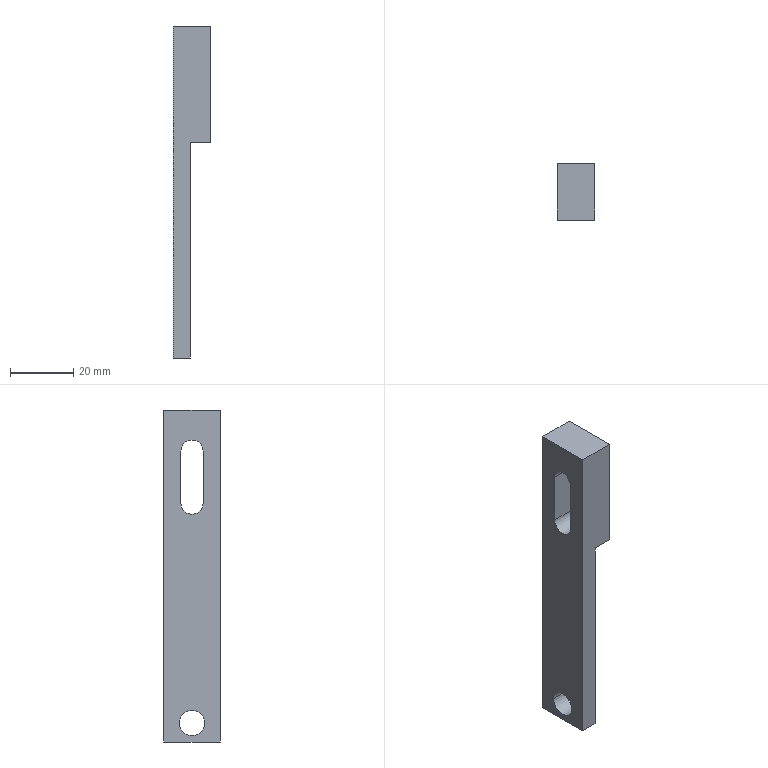Part | NX | 1 solid | 14 faces | box 12 x 18 x 105 mm | volume 12588 mm3 | plane 10 | cylinder 4 | commonest cylinder face diameters 7 x2 8 x2
STEP:
#1=CARTESIAN_POINT('',(-203.,42.75,26.5));
#2=VERTEX_POINT('',#1);
#3=CARTESIAN_POINT('',(-203.,60.75,26.5));
#4=VERTEX_POINT('',#3);
#5=CARTESIAN_POINT('',(-203.,53.935,26.5));
#6=DIRECTION('',(0.,1.,0.));
#7=VECTOR('',#6,1000.);
#8=LINE('',#5,#7);
#9=EDGE_CURVE('',#2,#4,#8,.T.);
#10=ORIENTED_EDGE('',*,*,#9,.T.);
#11=CARTESIAN_POINT('',(-215.,60.75,26.5));
#12=VERTEX_POINT('',#11);
#13=CARTESIAN_POINT('',(-203.,60.75,26.5));
#14=DIRECTION('',(1.,0.,0.));
#15=VECTOR('',#14,1000.);
#16=LINE('',#13,#15);
#17=EDGE_CURVE('',#12,#4,#16,.T.);
#18=ORIENTED_EDGE('',*,*,#17,.F.);
#19=CARTESIAN_POINT('',(-215.,42.75,26.5));
#20=VERTEX_POINT('',#19);
#21=CARTESIAN_POINT('',(-215.,53.935,26.5));
#22=DIRECTION('',(0.,-1.,0.));
#23=VECTOR('',#22,1000.);
#24=LINE('',#21,#23);
#25=EDGE_CURVE('',#12,#20,#24,.T.);
#26=ORIENTED_EDGE('',*,*,#25,.T.);
#27=CARTESIAN_POINT('',(-203.,42.75,26.5));
#28=DIRECTION('',(-1.,0.,0.));
#29=VECTOR('',#28,1000.);
#30=LINE('',#27,#29);
#31=EDGE_CURVE('',#2,#20,#30,.T.);
#32=ORIENTED_EDGE('',*,*,#31,.F.);
#33=EDGE_LOOP('',(#10,#18,#26,#32));
#34=FACE_BOUND('',#33,.T.);
#35=CARTESIAN_POINT('',(-203.,60.75,26.5));
#36=DIRECTION('',(0.,0.,1.));
#37=DIRECTION('',(1.,0.,0.));
#38=AXIS2_PLACEMENT_3D('',#35,#36,#37);
#39=PLANE('',#38);
#40=ADVANCED_FACE('',(#34),#39,.T.);
#41=CARTESIAN_POINT('',(-215.,60.75,-78.5));
#42=VERTEX_POINT('',#41);
#43=CARTESIAN_POINT('',(-215.,60.75,10.132));
#44=DIRECTION('',(0.,0.,1.));
#45=VECTOR('',#44,1000.);
#46=LINE('',#43,#45);
#47=EDGE_CURVE('',#42,#12,#46,.T.);
#48=ORIENTED_EDGE('',*,*,#47,.T.);
#49=ORIENTED_EDGE('',*,*,#17,.T.);
#50=CARTESIAN_POINT('',(-203.,60.75,-10.4));
#51=VERTEX_POINT('',#50);
#52=CARTESIAN_POINT('',(-203.,60.75,10.132));
#53=DIRECTION('',(0.,0.,-1.));
#54=VECTOR('',#53,1000.);
#55=LINE('',#52,#54);
#56=EDGE_CURVE('',#4,#51,#55,.T.);
#57=ORIENTED_EDGE('',*,*,#56,.T.);
#58=CARTESIAN_POINT('',(-209.5,60.75,-10.4));
#59=VERTEX_POINT('',#58);
#60=CARTESIAN_POINT('',(-203.,60.75,-10.4));
#61=DIRECTION('',(1.,0.,0.));
#62=VECTOR('',#61,1000.);
#63=LINE('',#60,#62);
#64=EDGE_CURVE('',#59,#51,#63,.T.);
#65=ORIENTED_EDGE('',*,*,#64,.F.);
#66=CARTESIAN_POINT('',(-209.5,60.75,-78.5));
#67=VERTEX_POINT('',#66);
#68=CARTESIAN_POINT('',(-209.5,60.75,10.132));
#69=DIRECTION('',(0.,0.,1.));
#70=VECTOR('',#69,1000.);
#71=LINE('',#68,#70);
#72=EDGE_CURVE('',#67,#59,#71,.T.);
#73=ORIENTED_EDGE('',*,*,#72,.F.);
#74=CARTESIAN_POINT('',(-203.,60.75,-78.5));
#75=DIRECTION('',(-1.,0.,0.));
#76=VECTOR('',#75,1000.);
#77=LINE('',#74,#76);
#78=EDGE_CURVE('',#67,#42,#77,.T.);
#79=ORIENTED_EDGE('',*,*,#78,.T.);
#80=EDGE_LOOP('',(#48,#49,#57,#65,#73,#79));
#81=FACE_BOUND('',#80,.T.);
#82=CARTESIAN_POINT('',(-203.,60.75,0.5));
#83=DIRECTION('',(0.,1.,0.));
#84=DIRECTION('',(1.,0.,0.));
#85=AXIS2_PLACEMENT_3D('',#82,#83,#84);
#86=PLANE('',#85);
#87=ADVANCED_FACE('',(#81),#86,.T.);
#88=CARTESIAN_POINT('',(-215.,42.75,-78.5));
#89=VERTEX_POINT('',#88);
#90=CARTESIAN_POINT('',(-215.,53.935,-78.5));
#91=DIRECTION('',(0.,1.,0.));
#92=VECTOR('',#91,1000.);
#93=LINE('',#90,#92);
#94=EDGE_CURVE('',#89,#42,#93,.T.);
#95=ORIENTED_EDGE('',*,*,#94,.T.);
#96=ORIENTED_EDGE('',*,*,#78,.F.);
#97=CARTESIAN_POINT('',(-209.5,42.75,-78.5));
#98=VERTEX_POINT('',#97);
#99=CARTESIAN_POINT('',(-209.5,53.935,-78.5));
#100=DIRECTION('',(0.,1.,0.));
#101=VECTOR('',#100,1000.);
#102=LINE('',#99,#101);
#103=EDGE_CURVE('',#98,#67,#102,.T.);
#104=ORIENTED_EDGE('',*,*,#103,.F.);
#105=CARTESIAN_POINT('',(-203.,42.75,-78.5));
#106=DIRECTION('',(1.,0.,0.));
#107=VECTOR('',#106,1000.);
#108=LINE('',#105,#107);
#109=EDGE_CURVE('',#89,#98,#108,.T.);
#110=ORIENTED_EDGE('',*,*,#109,.F.);
#111=EDGE_LOOP('',(#95,#96,#104,#110));
#112=FACE_BOUND('',#111,.T.);
#113=CARTESIAN_POINT('',(-203.,42.75,-78.5));
#114=DIRECTION('',(0.,0.,-1.));
#115=DIRECTION('',(0.,-1.,0.));
#116=AXIS2_PLACEMENT_3D('',#113,#114,#115);
#117=PLANE('',#116);
#118=ADVANCED_FACE('',(#112),#117,.T.);
#119=CARTESIAN_POINT('',(-203.,42.75,-10.4));
#120=VERTEX_POINT('',#119);
#121=CARTESIAN_POINT('',(-209.5,42.75,-10.4));
#122=VERTEX_POINT('',#121);
#123=CARTESIAN_POINT('',(-203.,42.75,-10.4));
#124=DIRECTION('',(-1.,0.,0.));
#125=VECTOR('',#124,1000.);
#126=LINE('',#123,#125);
#127=EDGE_CURVE('',#120,#122,#126,.T.);
#128=ORIENTED_EDGE('',*,*,#127,.F.);
#129=CARTESIAN_POINT('',(-203.,42.75,10.132));
#130=DIRECTION('',(0.,0.,1.));
#131=VECTOR('',#130,1000.);
#132=LINE('',#129,#131);
#133=EDGE_CURVE('',#120,#2,#132,.T.);
#134=ORIENTED_EDGE('',*,*,#133,.T.);
#135=ORIENTED_EDGE('',*,*,#31,.T.);
#136=CARTESIAN_POINT('',(-215.,42.75,10.132));
#137=DIRECTION('',(0.,0.,-1.));
#138=VECTOR('',#137,1000.);
#139=LINE('',#136,#138);
#140=EDGE_CURVE('',#20,#89,#139,.T.);
#141=ORIENTED_EDGE('',*,*,#140,.T.);
#142=ORIENTED_EDGE('',*,*,#109,.T.);
#143=CARTESIAN_POINT('',(-209.5,42.75,10.132));
#144=DIRECTION('',(0.,0.,-1.));
#145=VECTOR('',#144,1000.);
#146=LINE('',#143,#145);
#147=EDGE_CURVE('',#122,#98,#146,.T.);
#148=ORIENTED_EDGE('',*,*,#147,.F.);
#149=EDGE_LOOP('',(#128,#134,#135,#141,#142,#148));
#150=FACE_BOUND('',#149,.T.);
#151=CARTESIAN_POINT('',(-203.,42.75,18.5));
#152=DIRECTION('',(0.,-1.,0.));
#153=DIRECTION('',(0.,0.,-1.));
#154=AXIS2_PLACEMENT_3D('',#151,#152,#153);
#155=PLANE('',#154);
#156=ADVANCED_FACE('',(#150),#155,.T.);
#157=CARTESIAN_POINT('',(-209.5,55.75,-72.5));
#158=VERTEX_POINT('',#157);
#159=CARTESIAN_POINT('',(-209.5,47.75,-72.5));
#160=VERTEX_POINT('',#159);
#161=CARTESIAN_POINT('',(-209.5,51.75,-72.5));
#162=DIRECTION('',(-1.,0.,0.));
#163=DIRECTION('',(0.,-1.,0.));
#164=AXIS2_PLACEMENT_3D('',#161,#162,#163);
#165=CIRCLE('',#164,4.);
#166=EDGE_CURVE('',#158,#160,#165,.T.);
#167=ORIENTED_EDGE('',*,*,#166,.F.);
#168=CARTESIAN_POINT('',(-215.,55.75,-72.5));
#169=VERTEX_POINT('',#168);
#170=CARTESIAN_POINT('',(-202.,55.75,-72.5));
#171=DIRECTION('',(-1.,0.,0.));
#172=VECTOR('',#171,1000.);
#173=LINE('',#170,#172);
#174=EDGE_CURVE('',#169,#158,#173,.F.);
#175=ORIENTED_EDGE('',*,*,#174,.F.);
#176=CARTESIAN_POINT('',(-215.,47.75,-72.5));
#177=VERTEX_POINT('',#176);
#178=CARTESIAN_POINT('',(-215.,51.75,-72.5));
#179=DIRECTION('',(-1.,0.,0.));
#180=DIRECTION('',(0.,-1.,0.));
#181=AXIS2_PLACEMENT_3D('',#178,#179,#180);
#182=CIRCLE('',#181,4.);
#183=EDGE_CURVE('',#169,#177,#182,.T.);
#184=ORIENTED_EDGE('',*,*,#183,.T.);
#185=CARTESIAN_POINT('',(-202.,47.75,-72.5));
#186=DIRECTION('',(-1.,0.,0.));
#187=VECTOR('',#186,1000.);
#188=LINE('',#185,#187);
#189=EDGE_CURVE('',#177,#160,#188,.F.);
#190=ORIENTED_EDGE('',*,*,#189,.T.);
#191=EDGE_LOOP('',(#167,#175,#184,#190));
#192=FACE_BOUND('',#191,.T.);
#193=CARTESIAN_POINT('',(-202.,51.75,-72.5));
#194=DIRECTION('',(-1.,0.,0.));
#195=DIRECTION('',(0.,-1.,0.));
#196=AXIS2_PLACEMENT_3D('',#193,#194,#195);
#197=CYLINDRICAL_SURFACE('',#196,4.);
#198=ADVANCED_FACE('',(#192),#197,.F.);
#199=ORIENTED_EDGE('',*,*,#147,.T.);
#200=ORIENTED_EDGE('',*,*,#103,.T.);
#201=ORIENTED_EDGE('',*,*,#72,.T.);
#202=CARTESIAN_POINT('',(-209.5,53.935,-10.4));
#203=DIRECTION('',(0.,-1.,0.));
#204=VECTOR('',#203,1000.);
#205=LINE('',#202,#204);
#206=EDGE_CURVE('',#59,#122,#205,.T.);
#207=ORIENTED_EDGE('',*,*,#206,.T.);
#208=EDGE_LOOP('',(#199,#200,#201,#207));
#209=FACE_BOUND('',#208,.T.);
#210=ORIENTED_EDGE('',*,*,#166,.T.);
#211=CARTESIAN_POINT('',(-209.5,51.75,-72.5));
#212=DIRECTION('',(-1.,0.,0.));
#213=DIRECTION('',(0.,-1.,0.));
#214=AXIS2_PLACEMENT_3D('',#211,#212,#213);
#215=CIRCLE('',#214,4.);
#216=EDGE_CURVE('',#160,#158,#215,.T.);
#217=ORIENTED_EDGE('',*,*,#216,.T.);
#218=EDGE_LOOP('',(#210,#217));
#219=FACE_BOUND('',#218,.T.);
#220=CARTESIAN_POINT('',(-209.5,40.95,-13.4));
#221=DIRECTION('',(-1.,0.,0.));
#222=DIRECTION('',(0.,0.,1.));
#223=AXIS2_PLACEMENT_3D('',#220,#221,#222);
#224=PLANE('',#223);
#225=ADVANCED_FACE('',(#209,#219),#224,.F.);
#226=CARTESIAN_POINT('',(-215.,55.25,-3.));
#227=VERTEX_POINT('',#226);
#228=CARTESIAN_POINT('',(-215.,48.25,-3.));
#229=VERTEX_POINT('',#228);
#230=CARTESIAN_POINT('',(-215.,51.75,-3.));
#231=DIRECTION('',(-1.,0.,0.));
#232=DIRECTION('',(0.,-1.,0.));
#233=AXIS2_PLACEMENT_3D('',#230,#231,#232);
#234=CIRCLE('',#233,3.5);
#235=EDGE_CURVE('',#227,#229,#234,.T.);
#236=ORIENTED_EDGE('',*,*,#235,.T.);
#237=CARTESIAN_POINT('',(-203.,48.25,-3.));
#238=VERTEX_POINT('',#237);
#239=CARTESIAN_POINT('',(-201.8,48.25,-3.));
#240=DIRECTION('',(-1.,0.,0.));
#241=VECTOR('',#240,1000.);
#242=LINE('',#239,#241);
#243=EDGE_CURVE('',#238,#229,#242,.T.);
#244=ORIENTED_EDGE('',*,*,#243,.F.);
#245=CARTESIAN_POINT('',(-203.,55.25,-3.));
#246=VERTEX_POINT('',#245);
#247=CARTESIAN_POINT('',(-203.,51.75,-3.));
#248=DIRECTION('',(-1.,0.,0.));
#249=DIRECTION('',(0.,-1.,0.));
#250=AXIS2_PLACEMENT_3D('',#247,#248,#249);
#251=CIRCLE('',#250,3.5);
#252=EDGE_CURVE('',#246,#238,#251,.T.);
#253=ORIENTED_EDGE('',*,*,#252,.F.);
#254=CARTESIAN_POINT('',(-201.8,55.25,-3.));
#255=DIRECTION('',(-1.,0.,0.));
#256=VECTOR('',#255,1000.);
#257=LINE('',#254,#256);
#258=EDGE_CURVE('',#246,#227,#257,.T.);
#259=ORIENTED_EDGE('',*,*,#258,.T.);
#260=EDGE_LOOP('',(#236,#244,#253,#259));
#261=FACE_BOUND('',#260,.T.);
#262=CARTESIAN_POINT('',(-201.8,51.75,-3.));
#263=DIRECTION('',(-1.,0.,0.));
#264=DIRECTION('',(0.,-1.,0.));
#265=AXIS2_PLACEMENT_3D('',#262,#263,#264);
#266=CYLINDRICAL_SURFACE('',#265,3.5);
#267=ADVANCED_FACE('',(#261),#266,.F.);
#268=ORIENTED_EDGE('',*,*,#189,.F.);
#269=CARTESIAN_POINT('',(-215.,51.75,-72.5));
#270=DIRECTION('',(-1.,0.,0.));
#271=DIRECTION('',(0.,-1.,0.));
#272=AXIS2_PLACEMENT_3D('',#269,#270,#271);
#273=CIRCLE('',#272,4.);
#274=EDGE_CURVE('',#177,#169,#273,.T.);
#275=ORIENTED_EDGE('',*,*,#274,.T.);
#276=ORIENTED_EDGE('',*,*,#174,.T.);
#277=ORIENTED_EDGE('',*,*,#216,.F.);
#278=EDGE_LOOP('',(#268,#275,#276,#277));
#279=FACE_BOUND('',#278,.T.);
#280=CARTESIAN_POINT('',(-202.,51.75,-72.5));
#281=DIRECTION('',(-1.,0.,0.));
#282=DIRECTION('',(0.,-1.,0.));
#283=AXIS2_PLACEMENT_3D('',#280,#281,#282);
#284=CYLINDRICAL_SURFACE('',#283,4.);
#285=ADVANCED_FACE('',(#279),#284,.F.);
#286=ORIENTED_EDGE('',*,*,#140,.F.);
#287=ORIENTED_EDGE('',*,*,#25,.F.);
#288=ORIENTED_EDGE('',*,*,#47,.F.);
#289=ORIENTED_EDGE('',*,*,#94,.F.);
#290=EDGE_LOOP('',(#286,#287,#288,#289));
#291=FACE_BOUND('',#290,.T.);
#292=CARTESIAN_POINT('',(-215.,48.25,13.5));
#293=VERTEX_POINT('',#292);
#294=CARTESIAN_POINT('',(-215.,48.25,10.132));
#295=DIRECTION('',(0.,0.,1.));
#296=VECTOR('',#295,1000.);
#297=LINE('',#294,#296);
#298=EDGE_CURVE('',#229,#293,#297,.T.);
#299=ORIENTED_EDGE('',*,*,#298,.F.);
#300=ORIENTED_EDGE('',*,*,#235,.F.);
#301=CARTESIAN_POINT('',(-215.,55.25,13.5));
#302=VERTEX_POINT('',#301);
#303=CARTESIAN_POINT('',(-215.,55.25,10.132));
#304=DIRECTION('',(0.,0.,-1.));
#305=VECTOR('',#304,1000.);
#306=LINE('',#303,#305);
#307=EDGE_CURVE('',#302,#227,#306,.T.);
#308=ORIENTED_EDGE('',*,*,#307,.F.);
#309=CARTESIAN_POINT('',(-215.,51.75,13.5));
#310=DIRECTION('',(-1.,0.,0.));
#311=DIRECTION('',(0.,-1.,0.));
#312=AXIS2_PLACEMENT_3D('',#309,#310,#311);
#313=CIRCLE('',#312,3.5);
#314=EDGE_CURVE('',#293,#302,#313,.T.);
#315=ORIENTED_EDGE('',*,*,#314,.F.);
#316=EDGE_LOOP('',(#299,#300,#308,#315));
#317=FACE_BOUND('',#316,.T.);
#318=ORIENTED_EDGE('',*,*,#183,.F.);
#319=ORIENTED_EDGE('',*,*,#274,.F.);
#320=EDGE_LOOP('',(#318,#319));
#321=FACE_BOUND('',#320,.T.);
#322=CARTESIAN_POINT('',(-215.,53.935,10.132));
#323=DIRECTION('',(-1.,0.,0.));
#324=DIRECTION('',(0.,0.,1.));
#325=AXIS2_PLACEMENT_3D('',#322,#323,#324);
#326=PLANE('',#325);
#327=ADVANCED_FACE('',(#291,#317,#321),#326,.T.);
#328=CARTESIAN_POINT('',(-203.,48.25,13.5));
#329=VERTEX_POINT('',#328);
#330=CARTESIAN_POINT('',(-203.,55.25,13.5));
#331=VERTEX_POINT('',#330);
#332=CARTESIAN_POINT('',(-203.,51.75,13.5));
#333=DIRECTION('',(-1.,0.,0.));
#334=DIRECTION('',(0.,-1.,0.));
#335=AXIS2_PLACEMENT_3D('',#332,#333,#334);
#336=CIRCLE('',#335,3.5);
#337=EDGE_CURVE('',#329,#331,#336,.T.);
#338=ORIENTED_EDGE('',*,*,#337,.F.);
#339=CARTESIAN_POINT('',(-203.,48.25,13.5));
#340=DIRECTION('',(-1.,0.,0.));
#341=VECTOR('',#340,1000.);
#342=LINE('',#339,#341);
#343=EDGE_CURVE('',#329,#293,#342,.T.);
#344=ORIENTED_EDGE('',*,*,#343,.T.);
#345=ORIENTED_EDGE('',*,*,#314,.T.);
#346=CARTESIAN_POINT('',(-203.,55.25,13.5));
#347=DIRECTION('',(-1.,0.,0.));
#348=VECTOR('',#347,1000.);
#349=LINE('',#346,#348);
#350=EDGE_CURVE('',#331,#302,#349,.T.);
#351=ORIENTED_EDGE('',*,*,#350,.F.);
#352=EDGE_LOOP('',(#338,#344,#345,#351));
#353=FACE_BOUND('',#352,.T.);
#354=CARTESIAN_POINT('',(-202.,51.75,13.5));
#355=DIRECTION('',(-1.,0.,0.));
#356=DIRECTION('',(0.,-1.,0.));
#357=AXIS2_PLACEMENT_3D('',#354,#355,#356);
#358=CYLINDRICAL_SURFACE('',#357,3.5);
#359=ADVANCED_FACE('',(#353),#358,.F.);
#360=CARTESIAN_POINT('',(-203.,55.25,10.132));
#361=DIRECTION('',(0.,0.,-1.));
#362=VECTOR('',#361,1000.);
#363=LINE('',#360,#362);
#364=EDGE_CURVE('',#331,#246,#363,.T.);
#365=ORIENTED_EDGE('',*,*,#364,.F.);
#366=ORIENTED_EDGE('',*,*,#350,.T.);
#367=ORIENTED_EDGE('',*,*,#307,.T.);
#368=ORIENTED_EDGE('',*,*,#258,.F.);
#369=EDGE_LOOP('',(#365,#366,#367,#368));
#370=FACE_BOUND('',#369,.T.);
#371=CARTESIAN_POINT('',(-202.,55.25,5.5));
#372=DIRECTION('',(0.,1.,0.));
#373=DIRECTION('',(1.,0.,0.));
#374=AXIS2_PLACEMENT_3D('',#371,#372,#373);
#375=PLANE('',#374);
#376=ADVANCED_FACE('',(#370),#375,.F.);
#377=ORIENTED_EDGE('',*,*,#127,.T.);
#378=ORIENTED_EDGE('',*,*,#206,.F.);
#379=ORIENTED_EDGE('',*,*,#64,.T.);
#380=CARTESIAN_POINT('',(-203.,53.935,-10.4));
#381=DIRECTION('',(0.,1.,0.));
#382=VECTOR('',#381,1000.);
#383=LINE('',#380,#382);
#384=EDGE_CURVE('',#120,#51,#383,.T.);
#385=ORIENTED_EDGE('',*,*,#384,.F.);
#386=EDGE_LOOP('',(#377,#378,#379,#385));
#387=FACE_BOUND('',#386,.T.);
#388=CARTESIAN_POINT('',(-203.,40.95,-10.4));
#389=DIRECTION('',(0.,0.,1.));
#390=DIRECTION('',(1.,0.,0.));
#391=AXIS2_PLACEMENT_3D('',#388,#389,#390);
#392=PLANE('',#391);
#393=ADVANCED_FACE('',(#387),#392,.F.);
#394=ORIENTED_EDGE('',*,*,#298,.T.);
#395=ORIENTED_EDGE('',*,*,#343,.F.);
#396=CARTESIAN_POINT('',(-203.,48.25,10.132));
#397=DIRECTION('',(0.,0.,1.));
#398=VECTOR('',#397,1000.);
#399=LINE('',#396,#398);
#400=EDGE_CURVE('',#238,#329,#399,.T.);
#401=ORIENTED_EDGE('',*,*,#400,.F.);
#402=ORIENTED_EDGE('',*,*,#243,.T.);
#403=EDGE_LOOP('',(#394,#395,#401,#402));
#404=FACE_BOUND('',#403,.T.);
#405=CARTESIAN_POINT('',(-201.8,48.25,13.5));
#406=DIRECTION('',(0.,-1.,0.));
#407=DIRECTION('',(0.,0.,-1.));
#408=AXIS2_PLACEMENT_3D('',#405,#406,#407);
#409=PLANE('',#408);
#410=ADVANCED_FACE('',(#404),#409,.F.);
#411=ORIENTED_EDGE('',*,*,#384,.T.);
#412=ORIENTED_EDGE('',*,*,#56,.F.);
#413=ORIENTED_EDGE('',*,*,#9,.F.);
#414=ORIENTED_EDGE('',*,*,#133,.F.);
#415=EDGE_LOOP('',(#411,#412,#413,#414));
#416=FACE_BOUND('',#415,.T.);
#417=ORIENTED_EDGE('',*,*,#400,.T.);
#418=ORIENTED_EDGE('',*,*,#337,.T.);
#419=ORIENTED_EDGE('',*,*,#364,.T.);
#420=ORIENTED_EDGE('',*,*,#252,.T.);
#421=EDGE_LOOP('',(#417,#418,#419,#420));
#422=FACE_BOUND('',#421,.T.);
#423=CARTESIAN_POINT('',(-203.,53.935,10.132));
#424=DIRECTION('',(-1.,0.,0.));
#425=DIRECTION('',(0.,0.,1.));
#426=AXIS2_PLACEMENT_3D('',#423,#424,#425);
#427=PLANE('',#426);
#428=ADVANCED_FACE('',(#416,#422),#427,.F.);
#429=CLOSED_SHELL('',(#40,#87,#118,#156,#198,#225,#267,#285,#327,#359,#376,#393,#410,#428));
#430=MANIFOLD_SOLID_BREP('',#429);
#431=(LENGTH_UNIT()NAMED_UNIT(*)SI_UNIT(.MILLI.,.METRE.));
#432=UNCERTAINTY_MEASURE_WITH_UNIT(LENGTH_MEASURE(0.00001),#431,'','');
#433=(NAMED_UNIT(*)PLANE_ANGLE_UNIT()SI_UNIT($,.RADIAN.));
#434=(NAMED_UNIT(*)SI_UNIT($,.STERADIAN.)SOLID_ANGLE_UNIT());
#435=(GEOMETRIC_REPRESENTATION_CONTEXT(3)GLOBAL_UNCERTAINTY_ASSIGNED_CONTEXT((#432))GLOBAL_UNIT_ASSIGNED_CONTEXT((#431,#433,#434))REPRESENTATION_CONTEXT('',''));
#436=ADVANCED_BREP_SHAPE_REPRESENTATION('',(#430),#435);